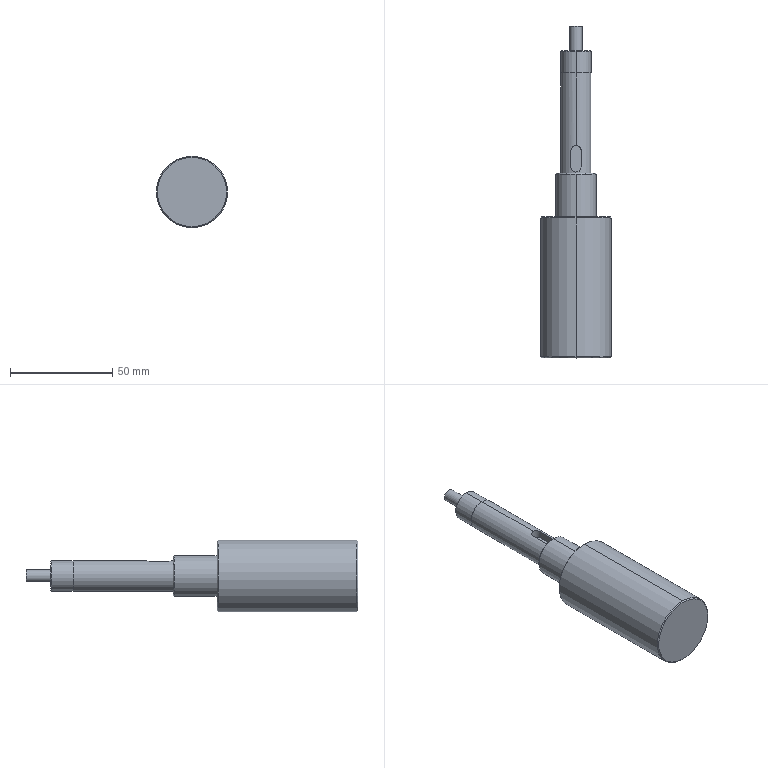Part | STEP file | ND25021-01-JDKMJ-06-TL | 1 solid | 29 faces | box 35 x 162.5 x 35 mm | volume 83750 mm3 | cylinder 11 | plane 10 | cone 8 | commonest cylinder face diameters 5 x2 14.8 x2 15 x2 20 x2 35 x2 6 x1